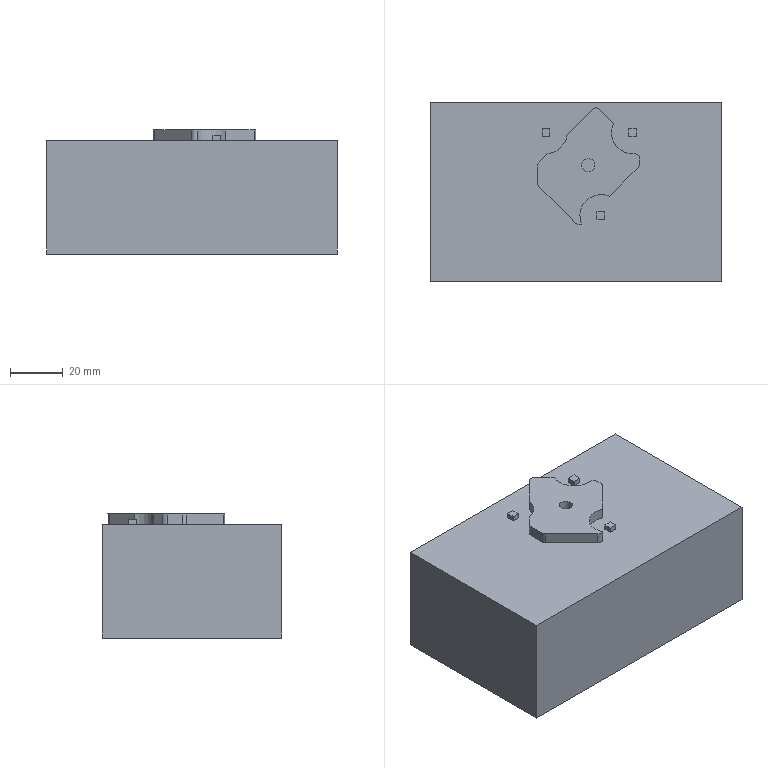CAM job | NX | 3-axis milling, drilling | part box 110.151 x 68.163 x 47.1 mm | stock box 110.151 x 68.163 x 47.1 mm
Tools:
number,name,description,diameter,corner_radius,flute_length,length,flutes
0,D50,Milling Tool-5 Parameters,50.0,0.0,50.0,75.0,2
0,D25R0,Milling Tool-5 Parameters,25.0,0.0,50.0,75.0,2
0,D6R0,Milling Tool-5 Parameters,6.0,0.0,40.0,40.0,2
12,D10R0,Milling Tool-5 Parameters,10.0,0.0,45.0,45.0,2
0,DK-Ø6,Drilling Tool,6.0,0.0,50.0,50.0,2
0,D1.8钻头,Drilling Tool,1.8,0.0,35.0,50.0,2
0,D2.75钻头,Drilling Tool,2.75,0.0,35.0,50.0,2
0,M2,Drilling Tool,2.0,0.0,35.0,50.0,4
0,M3,Drilling Tool,3.0,0.0,35.0,50.0,4
0,D16R0,Milling Tool-5 Parameters,16.0,0.0,50.0,75.0,2
0,D12R0,Milling Tool-5 Parameters,12.0,0.0,50.0,75.0,2
0,D4.2钻头,Drilling Tool,4.2,0.0,35.0,50.0,2
0,DK-Ø8,Countersink,8.0,0.0,0.0,60.0,2
0,D3.4钻头,Drilling Tool,3.4,0.0,35.0,50.0,2
0,M5,Drilling Tool,5.0,0.0,35.0,50.0,4
0,D4R0,Milling Tool-5 Parameters,4.0,0.0,50.0,75.0,2
4,D8R0,Milling Tool-5 Parameters,8.0,0.0,50.0,50.0,2
0,D2R0,Milling Tool-5 Parameters,2.0,0.0,20.0,20.0,2
0,R5,Milling Tool-Ball Mill,10.0,5.0,50.0,75.0,2
0,D3.7钻头,Drilling Tool,3.7,0.0,60.0,60.0,2
0,D5.3钻头,Drilling Tool,5.3,0.0,35.0,50.0,2
0,D3R0,Milling Tool-5 Parameters,3.0,0.0,28.0,28.0,2
0,DJ-Ø5,Countersink,5.0,0.0,0.0,60.0,2
0,DJ-Ø3,Countersink,3.0,0.0,0.0,20.0,2
0,DK-Ø12,Countersink,12.0,0.0,0.0,60.0,2
0,D8.5钻,Drilling Tool,8.5,0.0,35.0,50.0,2
0,D5.5钻,Drilling Tool,5.5,0.0,35.0,50.0,2
0,D6.6钻,Drilling Tool,6.5,0.0,35.0,50.0,2
0,D2.5钻,Drilling Tool,2.5,0.0,35.0,50.0,2
0,D05,Drilling Tool,5.0,0.0,35.0,50.0,2
0,M6,Drilling Tool,6.0,0.0,35.0,50.0,4
0,DK-Ø5,Countersink,5.0,0.0,0.0,60.0,2
0,D02钻头,Drilling Tool,2.0,0.0,35.0,80.0,2
0,M2.50,Drilling Tool,2.5,0.0,35.0,50.0,4
0,D2.5R0,Milling Tool-5 Parameters,2.5,0.0,50.0,75.0,2
0,D1.5R0,Milling Tool-5 Parameters,1.5,0.0,4.5,4.5,2
1,E63,Milling Tool-5 Parameters,63.0,0.0,50.0,75.0,2
0,DD10,Thread Mill,9.95,0.0,10.0,50.0,2
21,D10,Milling Tool-5 Parameters,10.0,0.0,50.0,75.0,2
Operations:
program,operation,operation_type,tool,method,geometry_group,spindle_rpm,surface_speed,feed_per_tooth,feed_cut,feed_plunge,cut_length_mm,path_length_mm,cut_time_min,machine_time_min
A01,FACE_MILLING,FaceMilling,E63,METHOD,MCS_MILL,3000.0,471.0,0.25,1500.0,100.0,413.956,579.956,0.276,0.3009
A01,PLANAR_PROFILE_2,PlanarMilling,E63,METHOD,MCS_MILL,5000.0,989.0,0.18,1800.0,100.0,3196.863,3424.863,1.776,1.807
A01,ZLEVEL_PROFILE_STEEP,ZLevelMilling,E63,METHOD,MCS_MILL,5000.0,100.0,0.1178,3000.0,100.0,8146.876,18371.908,2.716,4.073
A02,FACE_MILLING_1_COPY_1,FaceMilling,D25R0,METHOD,MCS_MILL,6000.0,392.0,0.25,2500.0,100.0,3268.899,3674.908,1.308,1.349
A02,PLANAR_MILL,PlanarMilling,D25R0,METHOD,MCS_MILL,6000.0,392.0,0.25,2500.0,100.0,4270.959,4460.559,1.708,1.736
A02,CAVITY_MILL_4,CavityMilling,D25R0,METHOD,MCS_MILL,6000.0,392.0,0.25,2500.0,100.0,3586.891,3906.091,1.435,1.479
A03,CAVITY_MILL_COPY_COPY,CavityMilling,D10R0,METHOD,MCS_MILL,5000.0,157.0,0.15,1500.0,100.0,915.845,1744.833,0.6106,0.763
A03,CAVITY_MILL,CavityMilling,D10R0,METHOD,MCS_MILL,5000.0,157.0,0.15,1500.0,100.0,1525.257,1761.257,1.017,1.068
A03,CAVITY_MILL_1,CavityMilling,D10R0,METHOD,MCS_MILL,4000.0,125.0,0.1875,1500.0,100.0,1369.169,1660.481,0.9128,0.9541
A04,DRILLING,Operation,DK-Ø8,METHOD,MCS_MILL,2000.0,37.0,0.05,200.0,0.0,12.0,469.097,0.06,0.1057
A04,DRILLING_COPY,Operation,DK-Ø8,METHOD,MCS_MILL,2000.0,37.0,0.05,200.0,0.0,12.0,548.039,0.06,0.1136
A04,DRILLING_COPY_COPY,Operation,DK-Ø8,METHOD,MCS_MILL,2000.0,37.0,0.05,200.0,0.0,6.7,302.057,0.0335,0.063
A04,DRILLING_COPY_COPY_COPY,Operation,DK-Ø8,METHOD,MCS_MILL,2000.0,37.0,0.05,200.0,0.0,11.4,521.628,0.057,0.108
A04,PLANAR_MILL_COPY,PlanarMilling,DK-Ø8,METHOD,MCS_MILL,3500.0,87.0,0.1714,1200.0,100.0,347.153,510.153,0.2893,0.3137
A05,DRILLING_COPY_COPY_COPY_COPY,Operation,D1.8钻头,METHOD,MCS_MILL,1800.0,10.0,0.0278,100.0,0.0,20.0,538.828,0.2,0.2519
A06,DRILLING_COPY_COPY_COPY_1,Operation,D2.75钻头,METHOD,MCS_MILL,2000.0,17.0,0.025,100.0,0.0,23.0,334.657,0.23,0.2612
A07,DRILLING_COPY_COPY_COPY_COPY_COPY,Operation,M2,METHOD,MCS_MILL,300.0,1.0,0.1,120.0,0.0,20.0,538.828,0.1667,0.2185
A08,DRILLING_COPY_COPY_COPY_COPY_COPY_COPY,Operation,M3,METHOD,MCS_MILL,300.0,2.0,0.125,150.0,0.0,17.0,322.657,0.1133,0.1439
A09,PLANAR_MILL_COPY_1,PlanarMilling,D10R0,METHOD,MCS_MILL,4000.0,125.0,0.1,800.0,100.0,369.021,555.321,0.4613,0.4892
B01,FACE_MILLING_COPY,FaceMilling,E63,METHOD,MCS_MILL,3500.0,692.0,0.3571,2500.0,100.0,3199.647,3711.185,1.28,1.339
B02,CAVITY_MILL_2,CavityMilling,D12R0,METHOD,MCS_MILL,5500.0,207.0,0.1364,1500.0,100.0,2703.853,2986.78,1.803,1.852
B03,PLANAR_MILL_2_COPY,PlanarMilling,D10R0,METHOD,MCS_MILL,4000.0,125.0,0.1,800.0,100.0,824.431,984.431,1.03,1.054
B03,CAVITY_MILL_2_COPY_1,CavityMilling,D10R0,METHOD,MCS_MILL,4500.0,141.0,0.0889,800.0,100.0,821.409,992.209,1.027,1.064
B04,DRILLING_COPY_COPY_COPY_COPY_1,Operation,DK-Ø8,METHOD,MCS_MILL,2000.0,37.0,0.05,200.0,0.0,11.1,457.326,0.0555,0.1001
B04,DRILLING_COPY_COPY_COPY_COPY_1_COPY_1,Operation,DK-Ø8,METHOD,MCS_MILL,2000.0,50.0,0.0375,150.0,0.0,18.0,560.039,0.12,0.1742
B04,PLANAR_MILL_COPY_COPY,PlanarMilling,DK-Ø8,METHOD,MCS_MILL,4000.0,100.0,0.15,1200.0,100.0,135.803,299.803,0.1132,0.1378
B04,PLANAR_MILL_COPY_COPY_COPY,PlanarMilling,DK-Ø8,METHOD,MCS_MILL,4000.0,100.0,0.15,1200.0,100.0,443.823,607.823,0.3699,0.3945
B04,DRILLING_COPY_COPY_COPY_COPY_1_COPY_2,Operation,DK-Ø8,METHOD,MCS_MILL,2000.0,37.0,0.05,200.0,0.0,8.4,310.48,0.042,0.0722
B05,DRILLING_COPY_COPY_COPY_COPY_1_COPY,Operation,D4.2钻头,METHOD,MCS_MILL,1800.0,23.0,0.0556,200.0,0.0,52.5,540.126,0.2625,0.3113
B05,DRILLING_COPY_COPY_COPY_COPY_1_COPY_COPY_2,Operation,D4.2钻头,METHOD,MCS_MILL,1800.0,23.0,0.0556,200.0,0.0,29.0,351.68,0.145,0.1773
B06,DRILLING_COPY_COPY_COPY_COPY_1_COPY_COPY,Operation,D3.4钻头,METHOD,MCS_MILL,1800.0,23.0,0.0556,200.0,0.0,30.0,584.039,0.15,0.2054
B07,DRILLING_COPY_COPY_COPY_COPY_1_COPY_COPY_1,Operation,M5,METHOD,MCS_MILL,400.0,6.0,0.2,320.0,0.0,43.5,522.126,0.1359,0.1838
B08,PLANAR_MILL_2,PlanarMilling,D4R0,METHOD,MCS_MILL,5000.0,62.0,0.15,1500.0,100.0,814.97,1251.944,0.5433,0.6029
B08,PLANAR_MILL_2_COPY_1,PlanarMilling,D4R0,METHOD,MCS_MILL,4000.0,50.0,0.025,200.0,100.0,31.176,479.723,0.1559,0.2183
B08,PLANAR_MILL_2_COPY_1_COPY,PlanarMilling,D4R0,METHOD,MCS_MILL,4000.0,50.0,0.025,200.0,100.0,31.176,479.723,0.1559,0.2183
B-5,PLANAR_MILL_2_COPY_COPY_1,PlanarMilling,D10R0,METHOD,MCS_MILL,4000.0,125.0,0.1,800.0,100.0,824.431,984.431,1.03,1.054
C01,DRILLING_1,Operation,DK-Ø5,METHOD,MCS_MILL,1500.0,23.0,0.05,150.0,0.0,4.0,108.0,0.0267,0.0371
C01,DRILLING_1_COPY,Operation,DK-Ø5,METHOD,MCS_MILL,1800.0,28.0,0.0417,150.0,0.0,3.5,107.0,0.0233,0.0337
C01,DRILLING_1_COPY_1,Operation,D3.7钻头,METHOD,MCS_MILL,1800.0,20.0,0.0417,150.0,0.0,22.5,145.0,0.15,0.1622
C01,DRILLING_1_COPY_COPY,Operation,D3.7钻头,METHOD,MCS_MILL,1800.0,20.0,0.0417,150.0,0.0,19.5,139.0,0.13,0.1419
C01,DRILLING_1_COPY_1_COPY,Operation,D5.3钻头,METHOD,MCS_MILL,1500.0,21.0,0.0667,200.0,0.0,11.5,123.0,0.0575,0.0687
C01,PLANAR_MILL_3_COPY_3,PlanarMilling,D8R0,METHOD,MCS_MILL,5000.0,125.0,0.1,1000.0,1500.0,239.323,604.823,0.2325,0.3
C01,PLANAR_MILL_3_COPY_3_COPY_2,PlanarMilling,D8R0,METHOD,MCS_MILL,5500.0,138.0,0.0909,1000.0,1500.0,70.885,686.617,0.0605,0.1839
C01,PLANAR_MILL_3_COPY_3_COPY,PlanarMilling,D8R0,METHOD,MCS_MILL,5500.0,138.0,0.0909,1000.0,1500.0,209.6,673.919,0.2027,0.2849
C01,PLANAR_MILL_3_COPY_3_COPY_COPY_1,PlanarMilling,D8R0,METHOD,MCS_MILL,5500.0,138.0,0.0909,1000.0,1500.0,209.6,673.919,0.2027,0.2849
C01,PLANAR_MILL_3_COPY_3_COPY_COPY,PlanarMilling,D8R0,METHOD,MCS_MILL,5500.0,138.0,0.0727,800.0,1500.0,104.8,340.319,0.1249,0.1698
C01,CAVITY_MILL_COPY_1_COPY,CavityMilling,D8R0,METHOD,MCS_MILL,5500.0,138.0,0.2273,2500.0,1500.0,2374.209,2588.138,0.9691,1.01
C01,PLANAR_PROFILE_COPY,PlanarMilling,D8R0,METHOD,MCS_MILL,5500.0,138.0,0.0909,1000.0,1500.0,79.287,154.488,0.0774,0.0887
C01,PLANAR_PROFILE_COPY_COPY,PlanarMilling,D8R0,METHOD,MCS_MILL,5500.0,138.0,0.0591,650.0,1500.0,91.316,166.516,0.1355,0.1468
C01,PLANAR_MILL_4,PlanarMilling,D6R0,METHOD,MCS_MILL,6500.0,122.0,0.1923,2500.0,100.0,723.805,899.003,0.2895,0.3151
C01,PLANAR_MILL_4_COPY,PlanarMilling,D6R0,METHOD,MCS_MILL,6500.0,122.0,0.0615,800.0,100.0,90.876,258.876,0.1136,0.1388
C01,PLANAR_MILL_3_COPY_3_COPY_COPY_COPY_COPY,PlanarMilling,D10,METHOD,MCS_MILL,3000.0,94.0,0.1333,800.0,1500.0,55.0,182.119,0.065,0.0925
C01,PLANAR_MILL_3_COPY_3_COPY_1,PlanarMilling,D10,METHOD,MCS_MILL,5000.0,125.0,0.1,1000.0,1500.0,86.159,221.459,0.0833,0.1126
C01,PLANAR_MILL_3_COPY_3_COPY_1_COPY_1,PlanarMilling,D10,METHOD,MCS_MILL,5000.0,125.0,0.1,1000.0,1500.0,86.159,221.459,0.0833,0.1126
C01,PLANAR_PROFILE_1,PlanarMilling,D10R0,METHOD,MCS_MILL,4500.0,141.0,0.0889,800.0,100.0,57.0,97.0,0.0713,0.0773
C01,PLANAR_PROFILE_1_COPY,PlanarMilling,D10R0,METHOD,MCS_MILL,4000.0,125.0,0.25,2000.0,100.0,676.096,1478.598,0.338,0.4314
C01,PLANAR_PROFILE_1_COPY_COPY,PlanarMilling,D10R0,METHOD,MCS_MILL,4000.0,125.0,0.05,400.0,100.0,67.498,186.298,0.3612,0.3791
C01,CAVITY_MILL_5,CavityMilling,D10R0,METHOD,MCS_MILL,4500.0,141.0,0.2222,2000.0,1000.0,2268.244,2661.886,1.298,1.347
C01,PLANAR_MILL_3_COPY_3_COPY_1_COPY,PlanarMilling,D10R0,METHOD,MCS_MILL,4000.0,125.0,0.1,800.0,100.0,49.615,173.471,0.062,0.0889
C01,CAVITY_MILL_COPY_1,CavityMilling,D10R0,METHOD,MCS_MILL,4000.0,125.0,0.1875,1500.0,100.0,953.266,2865.225,0.6355,0.9772
C01,FACE_MILLING_2,FaceMilling,D10R0,METHOD,MCS_MILL,4000.0,125.0,0.05,400.0,100.0,15.0,120.9,0.0375,0.0534
C01,PLANAR_MILL_3_COPY_4,PlanarMilling,D10R0,METHOD,MCS_MILL,4000.0,125.0,0.05,400.0,100.0,15.0,115.0,0.0375,0.0592
C01,PLANAR_MILL_3_COPY_4_COPY,PlanarMilling,D10R0,METHOD,MCS_MILL,4000.0,125.0,0.05,400.0,100.0,15.0,115.0,0.0375,0.0592
C01,PLANAR_MILL_3_COPY_4_COPY_COPY,PlanarMilling,D10R0,METHOD,MCS_MILL,4000.0,125.0,0.05,400.0,100.0,13.0,115.3,0.0325,0.0547
C01,PLANAR_MILL_3_COPY_3_COPY_COPY_1_COPY_COPY,PlanarMilling,R5,METHOD,MCS_MILL,4500.0,141.0,0.0444,400.0,1500.0,57.0,172.6,0.1288,0.1538
C01,CAVITY_MILL_COPY_1_COPY_COPY,CavityMilling,D4R0,METHOD,MCS_MILL,3000.0,37.0,0.25,1500.0,100.0,918.512,2163.766,0.6123,0.8259
C01,CAVITY_MILL_COPY_1_COPY_COPY_COPY,CavityMilling,D4R0,METHOD,MCS_MILL,3000.0,37.0,0.0667,400.0,100.0,94.513,223.713,0.2363,0.2643
C01,CAVITY_MILL_COPY_1_COPY_COPY_COPY_COPY,CavityMilling,D4R0,METHOD,MCS_MILL,3000.0,37.0,0.0667,400.0,100.0,94.513,223.713,0.2363,0.2643
C01,CAVITY_MILL_COPY_1_COPY_COPY_COPY_COPY_COPY,CavityMilling,D4R0,METHOD,MCS_MILL,3000.0,37.0,0.0667,400.0,100.0,94.513,223.713,0.2363,0.2643
C01,PLANAR_MILL_5,PlanarMilling,D3R0,METHOD,MCS_MILL,3500.0,32.0,0.2857,2000.0,100.0,1535.272,1640.072,0.7676,0.7831
C01,PLANAR_MILL_5_COPY,PlanarMilling,D3R0,METHOD,MCS_MILL,3000.0,28.0,0.25,1500.0,100.0,387.795,488.795,0.2585,0.2736
C01,PLANAR_MILL_5_COPY_COPY,PlanarMilling,D3R0,METHOD,MCS_MILL,3000.0,28.0,0.25,1500.0,100.0,1019.419,1125.119,0.6796,0.6952
C01,PLANAR_MILL_5_COPY_1,PlanarMilling,D3R0,METHOD,MCS_MILL,3000.0,28.0,0.05,300.0,100.0,128.642,233.542,0.4288,0.4445
C01,PLANAR_MILL_5_COPY_COPY_1,PlanarMilling,D3R0,METHOD,MCS_MILL,3000.0,28.0,0.05,300.0,100.0,129.768,230.868,0.4326,0.4477
C01,PLANAR_MILL_5_COPY_COPY_COPY_1,PlanarMilling,D3R0,METHOD,MCS_MILL,4000.0,37.0,0.05,400.0,100.0,101.608,204.608,0.254,0.2695
C01,PLANAR_MILL_5_COPY_COPY_COPY,PlanarMilling,D2R0,METHOD,MCS_MILL,5000.0,31.0,0.1,1000.0,100.0,313.795,1097.954,0.3138,0.4223
C01,PLANAR_MILL_5_COPY_2_COPY_2,PlanarMilling,DJ-Ø5,METHOD,MCS_MILL,4000.0,62.0,0.125,1000.0,100.0,132.795,296.795,0.1328,0.1574
C01,PLANAR_MILL_5_COPY_2_COPY,PlanarMilling,DJ-Ø5,METHOD,MCS_MILL,4000.0,62.0,0.125,1000.0,100.0,254.474,416.474,0.2545,0.2788
C01,PLANAR_MILL_5_COPY_2_COPY_COPY,PlanarMilling,DJ-Ø5,METHOD,MCS_MILL,4000.0,62.0,0.125,1000.0,100.0,21.283,183.283,0.0213,0.0456
C01,PLANAR_MILL_5_COPY_2_COPY_1,PlanarMilling,DJ-Ø5,METHOD,MCS_MILL,4000.0,62.0,0.125,1000.0,100.0,103.562,165.562,0.1036,0.1129
C01,PLANAR_MILL_5_COPY_2_COPY_COPY_COPY,PlanarMilling,DJ-Ø5,METHOD,MCS_MILL,4000.0,62.0,0.125,1000.0,100.0,40.053,281.928,0.0401,0.0744
C01,DRILLING_1_COPY_COPY_1,Operation,DJ-Ø5,METHOD,MCS_MILL,2000.0,31.0,0.025,100.0,0.0,12.4,573.031,0.124,0.1801
C01,DRILLING_1_COPY_COPY_3,Operation,DK-Ø5,METHOD,MCS_MILL,1800.0,28.0,0.0417,150.0,0.0,3.5,123.0,0.0233,0.0353
C01,PLANAR_MILL_3_COPY_5,PlanarMilling,D10R0,METHOD,MCS_MILL,4500.0,141.0,0.0667,600.0,1500.0,212.847,372.847,0.3443,0.379
C01,PLANAR_MILL_3_COPY_COPY,PlanarMilling,D10R0,METHOD,MCS_MILL,4500.0,141.0,0.0722,650.0,1500.0,99.417,265.417,0.1488,0.1848
C01,PLANAR_MILL_3_COPY_1_COPY_COPY,PlanarMilling,D10R0,METHOD,MCS_MILL,4500.0,141.0,0.0667,600.0,1500.0,196.762,359.922,0.3175,0.3529
C01,PLANAR_MILL_3_COPY_2_COPY_COPY,PlanarMilling,D10R0,METHOD,MCS_MILL,4500.0,141.0,0.0667,600.0,1500.0,184.007,356.007,0.2963,0.3335
C01,D10燕尾刀,PlanarMilling,D10R0,METHOD,MCS_MILL,6000.0,188.0,0.0667,800.0,100.0,197.01,358.698,0.2463,0.2704
C01,PLANAR_MILL_3_COPY_3_COPY_1_COPY_1_COPY,PlanarMilling,D8R0,METHOD,MCS_MILL,3500.0,87.0,0.0571,300.0,100.0,70.64,150.54,0.2355,0.2528
C01,THREAD_MILLING,ThreadMilling,DD10,METHOD,MCS_MILL,5000.0,155.0,0.04,400.0,100.0,485.462,652.491,1.214,1.23
C01,PLANAR_MILL_3,PlanarMilling,DJ-Ø3,METHOD,MCS_MILL,4000.0,37.0,0.1,800.0,100.0,120.498,278.498,0.1506,0.1664
C01,PLANAR_MILL_3_COPY,PlanarMilling,DJ-Ø3,METHOD,MCS_MILL,4000.0,37.0,0.1,800.0,100.0,114.233,272.233,0.1428,0.1586
C01,PLANAR_MILL_5_COPY_2_COPY_COPY_COPY_COPY,PlanarMilling,DJ-Ø3,METHOD,MCS_MILL,4000.0,37.0,0.05,400.0,100.0,210.599,312.799,0.5265,0.5418
C01,PLANAR_MILL_5_COPY_2_COPY_COPY_COPY_COPY_COPY,PlanarMilling,DJ-Ø3,METHOD,MCS_MILL,4000.0,37.0,0.05,400.0,100.0,107.962,210.162,0.2699,0.2852
C01,PLANAR_MILL_5_COPY_3_COPY_1,PlanarMilling,D3R0,METHOD,MCS_MILL,4000.0,37.0,0.05,400.0,100.0,221.318,392.745,0.5533,0.5784
C01,PLANAR_MILL_5_COPY_3_COPY_COPY,PlanarMilling,D3R0,METHOD,MCS_MILL,4000.0,37.0,0.05,400.0,100.0,174.956,343.956,0.4374,0.4623
C01,PLANAR_MILL_5_COPY_3_COPY_COPY_COPY_COPY_COPY,PlanarMilling,D3R0,METHOD,MCS_MILL,3000.0,28.0,0.0133,80.0,100.0,18.281,194.281,0.2285,0.2549
C01,PLANAR_MILL_5_COPY_3_COPY_1_COPY_1_COPY,PlanarMilling,D3R0,METHOD,MCS_MILL,3000.0,28.0,0.0133,80.0,100.0,18.306,201.159,0.2288,0.2563
C01,FLOOR_WALL_3_COPY_COPY_COPY,VolumeBased25DMillingOperation,D10R0,METHOD,MCS_MILL,3500.0,109.0,0.0857,600.0,100.0,1075.962,2001.095,1.793,1.911
C01,FLOOR_WALL_3_COPY_COPY,VolumeBased25DMillingOperation,D10R0,METHOD,MCS_MILL,3500.0,109.0,0.0857,600.0,100.0,1075.962,2009.083,1.793,1.912
C01,FACE_MILLING_2_COPY,FaceMilling,D10R0,METHOD,MCS_MILL,4000.0,125.0,0.125,1000.0,100.0,15.0,120.86,0.015,0.0309
C01,PLANAR_MILL_3_COPY_4_COPY_1_COPY,PlanarMilling,D10R0,METHOD,MCS_MILL,4500.0,141.0,0.0444,400.0,1500.0,15.0,115.0,0.0265,0.0482
C01,PLANAR_MILL_3_COPY_4_COPY_COPY_1_COPY,PlanarMilling,D10R0,METHOD,MCS_MILL,4500.0,141.0,0.0444,400.0,1500.0,15.0,115.0,0.0265,0.0482
C01,PLANAR_MILL_3_COPY_4_COPY_COPY_COPY_COPY_1,PlanarMilling,D10R0,METHOD,MCS_MILL,4500.0,141.0,0.0444,400.0,1500.0,13.0,115.34,0.0233,0.0455
C01,PLANAR_MILL_3_COPY_4_COPY_1_COPY_COPY,PlanarMilling,D10R0,METHOD,MCS_MILL,6500.0,204.0,0.0308,400.0,1500.0,15.0,115.0,0.0265,0.0482
C01,PLANAR_MILL_3_COPY_4_COPY_COPY_1_COPY_COPY,PlanarMilling,D10R0,METHOD,MCS_MILL,6500.0,204.0,0.0308,400.0,1500.0,15.0,115.0,0.0265,0.0482
C01,PLANAR_MILL_3_COPY_4_COPY_COPY_COPY_COPY_1_COPY_1,PlanarMilling,D10R0,METHOD,MCS_MILL,6500.0,204.0,0.0308,400.0,1500.0,13.0,115.36,0.0233,0.0455
C01,PLANAR_MILL_3_COPY_4_COPY_COPY_COPY_COPY_1_COPY,PlanarMilling,D10R0,METHOD,MCS_MILL,3000.0,94.0,0.1,600.0,1500.0,217.2,2345.48,0.302,0.7359
C01,PLANAR_MILL_3_COPY_4_COPY_COPY_COPY_COPY_COPY,PlanarMilling,D10R0,METHOD,MCS_MILL,3000.0,141.0,0.0667,600.0,1500.0,52.0,227.89,0.0817,0.1198
C01,PLANAR_MILL_3_COPY_4_COPY_COPY_COPY_COPY_COPY_COPY,PlanarMilling,D10R0,METHOD,MCS_MILL,3000.0,141.0,0.0667,600.0,1500.0,84.296,396.438,0.1305,0.185
D01,PLANAR_MILL_2_COPY_COPY,PlanarMilling,D10R0,METHOD,MCS_MILL,5000.0,157.0,0.2,2000.0,100.0,422.849,462.849,0.2114,0.2174
D01,PLANAR_MILL_2_COPY_COPY_COPY,PlanarMilling,D10R0,METHOD,MCS_MILL,5000.0,157.0,0.2,2000.0,100.0,63.946,103.946,0.032,0.038
D01,PLANAR_PROFILE,PlanarMilling,D10R0,METHOD,MCS_MILL,5000.0,157.0,0.2,2000.0,100.0,698.8,757,0.3494,0.3573
D01,PLANAR_PROFILE_COPY_2,PlanarMilling,D10R0,METHOD,MCS_MILL,5000.0,157.0,0.2,2000.0,100.0,1493.358,1551.558,0.7467,0.7546
D01,CAVITY_MILL_2_COPY,CavityMilling,D10R0,METHOD,MCS_MILL,5000.0,157.0,0.2,2000.0,100.0,712.062,757.062,0.356,0.3652
D01,CAVITY_MILL_2_COPY_COPY_COPY,CavityMilling,D10R0,METHOD,MCS_MILL,5000.0,157.0,0.2,2000.0,100.0,537.415,724.515,0.2687,0.3008
D01,PLANAR_MILL_COPY_1_1,PlanarMilling,D1.5R0,METHOD,MCS_MILL,6000.0,28.0,0.1,1200.0,100.0,982.84,1025.54,0.819,0.8253
D01,PLANAR_MILL_COPY_1_COPY,PlanarMilling,D1.5R0,METHOD,MCS_MILL,6000.0,33.0,0.0667,800.0,100.0,430.497,471.297,0.5381,0.5442
D01,PLANAR_MILL_1_1,PlanarMilling,D1.5R0,METHOD,MCS_MILL,6000.0,28.0,0.125,1500.0,100.0,3038.746,3711.707,2.026,2.101
D01,PLANAR_MILL_1_1_COPY,PlanarMilling,D1.5R0,METHOD,MCS_MILL,5500.0,25.0,0.0364,400.0,100.0,98.781,268.063,0.247,0.2723
D01,DRILLING_COPY_1,Operation,DK-Ø6,METHOD,MCS_MILL,2000.0,31.0,0.025,100.0,0.0,2.25,64.5,0.0225,0.0287
D01,DRILLING_COPY_1_COPY,Operation,DK-Ø6,METHOD,MCS_MILL,2000.0,31.0,0.025,100.0,0.0,2.25,64.5,0.0225,0.0287
D01,DRILLING_COPY_1_COPY_COPY_2,Operation,DK-Ø6,METHOD,MCS_MILL,2000.0,31.0,0.025,100.0,0.0,3.5,67.0,0.035,0.0414
D01,DRILLING_COPY_1_COPY_COPY_2_COPY,Operation,DK-Ø6,METHOD,MCS_MILL,2000.0,31.0,0.025,100.0,0.0,3.0,66.0,0.03,0.0363
D01,PLANAR_PROFILE_COPY_3,PlanarMilling,DK-Ø6,METHOD,MCS_MILL,4000.0,62.0,0.125,1000.0,100.0,381.698,423.698,0.3817,0.388
D01,PLANAR_PROFILE_COPY_3_COPY,PlanarMilling,DK-Ø6,METHOD,MCS_MILL,4000.0,62.0,0.125,1000.0,100.0,123.858,165.857,0.1239,0.1302
D01,PLANAR_PROFILE_COPY_3_COPY_COPY,PlanarMilling,DK-Ø6,METHOD,MCS_MILL,4000.0,62.0,0.125,1000.0,100.0,31.962,74.962,0.032,0.0384
D01,PLANAR_PROFILE_COPY_3_COPY_COPY_COPY,PlanarMilling,DK-Ø6,METHOD,MCS_MILL,4000.0,62.0,0.125,1000.0,100.0,24.5,67.5,0.0245,0.031
D01,PLANAR_PROFILE_COPY_3_COPY_COPY_1,PlanarMilling,DK-Ø6,METHOD,MCS_MILL,4000.0,62.0,0.125,1000.0,100.0,109.035,150.235,0.109,0.1152
D01,PLANAR_PROFILE_COPY_3_COPY_COPY_2,PlanarMilling,DK-Ø6,METHOD,MCS_MILL,4000.0,62.0,0.125,1000.0,100.0,40.142,81.142,0.0401,0.0463
D01,DRILLING_COPY_1_COPY_1,Operation,D02钻头,METHOD,MCS_MILL,1200.0,7.0,0.0417,100.0,0.0,31.0,122.0,0.31,0.3191
D01,DRILLING_COPY_1_COPY_COPY,Operation,D02钻头,METHOD,MCS_MILL,1200.0,7.0,0.0417,100.0,0.0,31.0,122.0,0.31,0.3191
D01,PLANAR_MILL_8,PlanarMilling,D2.5R0,METHOD,MCS_MILL,6000.0,47.0,0.0667,800.0,100.0,185.922,231.622,0.2324,0.2389
D01,PLANAR_MILL_COPY_2,PlanarMilling,D2.5R0,METHOD,MCS_MILL,6000.0,47.0,0.0417,500.0,100.0,59.901,101.341,0.1198,0.1259
D01,DRILLING_COPY_1_COPY_1_COPY,Operation,M2.50,METHOD,MCS_MILL,200.0,1.0,0.1125,90.0,0.0,6.0,72.0,0.0667,0.0733
D01,DRILLING_COPY_1_COPY_COPY_COPY,Operation,M2.50,METHOD,MCS_MILL,200.0,1.0,0.1125,90.0,0.0,6.0,72.0,0.0667,0.0733
D01,DRILLING_COPY_1_COPY_COPY_1,Operation,M5,METHOD,MCS_MILL,400.0,6.0,0.2,320.0,0.0,7.3,74.6,0.0228,0.0295
D01,PLANAR_MILL_2_COPY_COPY_COPY_1,PlanarMilling,D10R0,METHOD,MCS_MILL,5000.0,157.0,0.08,800.0,100.0,425.479,465.479,0.5318,0.5378
D01,PLANAR_MILL_2_COPY_COPY_COPY_COPY,PlanarMilling,D10R0,METHOD,MCS_MILL,4500.0,141.0,0.0889,800.0,100.0,60.946,100.946,0.0762,0.0822
D01,CAVITY_MILL_2_COPY_COPY_1_COPY_1,CavityMilling,D10R0,METHOD,MCS_MILL,4500.0,141.0,0.0889,800.0,100.0,1004.466,1217.66,1.256,1.29
D01,PLANAR_PROFILE_COPY_4,PlanarMilling,D10R0,METHOD,MCS_MILL,4500.0,141.0,0.0722,650.0,100.0,69.644,127.844,0.1071,0.1159
D01,PLANAR_PROFILE_COPY_2_COPY,PlanarMilling,D10R0,METHOD,MCS_MILL,4500.0,141.0,0.0722,650.0,100.0,148.864,207.065,0.229,0.2378
O0001.NC,PLANAR_MILL_2_COPY_COPY_COPY_2,PlanarMilling,D10R0,METHOD,MCS_MILL,5000.0,157.0,0.2,2000.0,100.0,422.849,462.849,0.2114,0.2174
O0001.NC,PLANAR_MILL_2_COPY_COPY_COPY_COPY_1,PlanarMilling,D10R0,METHOD,MCS_MILL,5000.0,157.0,0.2,2000.0,100.0,63.946,103.946,0.032,0.038
O0001.NC,PLANAR_PROFILE_COPY_1,PlanarMilling,D10R0,METHOD,MCS_MILL,5000.0,157.0,0.2,2000.0,100.0,698.015,756.215,0.349,0.3569
O0001.NC,PLANAR_PROFILE_COPY_2_COPY_1,PlanarMilling,D10R0,METHOD,MCS_MILL,5000.0,157.0,0.2,2000.0,100.0,1491.787,1549.987,0.7459,0.7538
O0001.NC,CAVITY_MILL_2_COPY_COPY,CavityMilling,D10R0,METHOD,MCS_MILL,5000.0,157.0,0.2,2000.0,100.0,712.062,757.062,0.356,0.3652
O0001.NC,CAVITY_MILL_2_COPY_COPY_COPY_COPY,CavityMilling,D10R0,METHOD,MCS_MILL,5000.0,157.0,0.2,2000.0,100.0,537.415,724.515,0.2687,0.3008
O0001.NC,PLANAR_MILL_2_COPY_COPY_COPY_1_COPY,PlanarMilling,D10R0,METHOD,MCS_MILL,5000.0,157.0,0.08,800.0,100.0,425.479,465.479,0.5318,0.5378
O0001.NC,PLANAR_MILL_2_COPY_COPY_COPY_COPY_COPY,PlanarMilling,D10R0,METHOD,MCS_MILL,4500.0,141.0,0.0889,800.0,100.0,60.946,100.946,0.0762,0.0822
O0001.NC,CAVITY_MILL_2_COPY_COPY_1_COPY_1_COPY,CavityMilling,D10R0,METHOD,MCS_MILL,4500.0,141.0,0.0889,800.0,100.0,1004.466,1217.66,1.256,1.29
O0001.NC,PLANAR_PROFILE_COPY_4_COPY,PlanarMilling,D10R0,METHOD,MCS_MILL,4500.0,141.0,0.0722,650.0,100.0,69.644,127.844,0.1071,0.1159
O0001.NC,PLANAR_PROFILE_COPY_2_COPY_COPY,PlanarMilling,D10R0,METHOD,MCS_MILL,4500.0,141.0,0.0722,650.0,100.0,148.864,207.065,0.229,0.2378
O0001.NC,PLANAR_PROFILE_COPY_3_COPY_COPY_3_COPY,PlanarMilling,D10R0,METHOD,MCS_MILL,4000.0,62.0,0.125,1000.0,100.0,83.897,134.097,0.0839,0.0914
O0001.NC,PLANAR_PROFILE_COPY_3_COPY_COPY_3_COPY_COPY,PlanarMilling,D10R0,METHOD,MCS_MILL,4000.0,62.0,0.125,800.0,100.0,83.897,134.097,0.1049,0.1124
O0001.NC,PLANAR_PROFILE_COPY_3_COPY_1,PlanarMilling,DK-Ø6,METHOD,MCS_MILL,4000.0,62.0,0.125,1000.0,100.0,381.698,423.698,0.3817,0.388
O0001.NC,PLANAR_PROFILE_COPY_3_COPY_COPY_3,PlanarMilling,DK-Ø6,METHOD,MCS_MILL,4000.0,62.0,0.125,1000.0,100.0,123.858,165.857,0.1239,0.1302
O0001.NC,PLANAR_PROFILE_COPY_3_COPY_COPY_COPY_1,PlanarMilling,DK-Ø6,METHOD,MCS_MILL,4000.0,62.0,0.125,1000.0,100.0,31.962,74.962,0.032,0.0384
O0001.NC,PLANAR_PROFILE_COPY_3_COPY_COPY_COPY_COPY,PlanarMilling,DK-Ø6,METHOD,MCS_MILL,4000.0,62.0,0.125,1000.0,100.0,24.5,67.5,0.0245,0.031
O0001.NC,DRILLING_COPY_1_COPY_2,Operation,DK-Ø6,METHOD,MCS_MILL,2000.0,31.0,0.025,100.0,0.0,4.5,194.427,0.045,0.064
1,FACE_MILLING_COPY_1,FaceMilling,D50,METHOD,MCS_MILL,3000.0,471.0,0.1667,1000.0,100.0,454.022,620.023,0.454,0.4789
1,PLANAR_MILL_1,PlanarMilling,D16R0,METHOD,MCS_MILL,4500.0,226.0,0.1667,1500.0,100.0,9544.266,10003.437,6.363,6.417
1,PLANAR_MILL_1_COPY,PlanarMilling,D16R0,METHOD,MCS_MILL,3500.0,175.0,0.0571,400.0,100.0,559.027,799.627,1.398,1.434
1,PLANAR_MILL_1_COPY_COPY,PlanarMilling,D16R0,METHOD,MCS_MILL,3500.0,175.0,0.0571,400.0,100.0,559.027,799.627,1.398,1.434
1,DRILLING_2,Operation,DK-Ø12,METHOD,NONE,2000.0,75.0,0.0375,150.0,0.0,24.0,597.151,0.16,0.2173
1,DRILLING_2_COPY,Operation,DK-Ø12,METHOD,NONE,2000.0,75.0,0.0375,150.0,0.0,21.0,442.484,0.14,0.1821
1,DRILLING_2_COPY_1,Operation,DK-Ø12,METHOD,NONE,2000.0,75.0,0.0375,150.0,0.0,12.0,259.212,0.08,0.1047
1,PLANAR_MILL_1_COPY_COPY_1,PlanarMilling,DK-Ø12,METHOD,MCS_MILL,3500.0,131.0,0.1714,1200.0,100.0,501.427,665.427,0.4179,0.4425
1,DRILLING_2_COPY_2,Operation,D8.5钻,METHOD,NONE,1500.0,40.0,0.05,150.0,0.0,146.0,841.151,0.9733,1.043
1,DRILLING_2_COPY_2_COPY,Operation,D8.5钻,METHOD,NONE,1500.0,40.0,0.05,150.0,0.0,61.5,513.442,0.41,0.4552
1,DRILLING_2_COPY_2_COPY_COPY,Operation,D5.5钻,METHOD,NONE,1500.0,40.0,0.05,150.0,0.0,135.0,660.442,0.9,0.9525
1,DRILLING_2_COPY_2_COPY_COPY_COPY,Operation,D5.5钻,METHOD,NONE,1500.0,40.0,0.05,150.0,0.0,34.0,303.212,0.2267,0.2536
1,DRILLING_2_COPY_2_COPY_COPY_1,Operation,D10R0,METHOD,NONE,1000.0,31.0,0.05,100.0,0.0,58.5,507.442,0.585,0.6299
1,PLANAR_MILL_1_COPY_1,PlanarMilling,D6R0,METHOD,MCS_MILL,5500.0,103.0,0.0727,800.0,100.0,807.102,1216.6,1.009,1.066
2,PLANAR_MILL_1_COPY_1_COPY,PlanarMilling,D6R0,METHOD,MCS_MILL,5500.0,103.0,0.0091,100.0,100.0,15.938,445.338,0.1594,0.2203
2,PLANAR_MILL_1_COPY_1_COPY_COPY,PlanarMilling,D6R0,METHOD,MCS_MILL,5500.0,103.0,0.0091,100.0,100.0,15.938,445.338,0.1594,0.2203
5,FACE_MILLING_COPY_1_COPY,FaceMilling,D50,METHOD,MCS_MILL,4500.0,706.0,0.3889,3500.0,100.0,454.022,624.423,0.1297,0.1553
5,FLOOR_WALL,VolumeBased25DMillingOperation,D16R0,METHOD,MCS_MILL,4500.0,226.0,0.2222,2000.0,100.0,2760.275,3404.434,1.38,1.461
5,FLOOR_WALL_1_COPY,VolumeBased25DMillingOperation,D16R0,METHOD,MCS_MILL,4500.0,226.0,0.1667,1500.0,100.0,942.016,1108.016,0.628,0.6529
5,FLOOR_WALL_COPY,VolumeBased25DMillingOperation,D16R0,METHOD,MCS_MILL,4500.0,226.0,0.0444,400.0,100.0,456.646,1000.453,1.142,1.214
5,FLOOR_WALL_1,VolumeBased25DMillingOperation,D16R0,METHOD,MCS_MILL,4500.0,226.0,0.0667,600.0,100.0,943.321,989.321,1.572,1.579
5,PLANAR_MILL_1_COPY_1_COPY_1_COPY_1,PlanarMilling,D6R0,METHOD,MCS_MILL,5500.0,103.0,0.0727,800.0,100.0,1659.041,2593.151,2.074,2.199
5,PLANAR_MILL_1_COPY_1_COPY_1_COPY_1_COPY,PlanarMilling,D6R0,METHOD,MCS_MILL,5500.0,103.0,0.0182,200.0,100.0,132.531,1106.857,0.6627,0.7961
5,PLANAR_MILL_1_COPY_COPY_1_COPY,PlanarMilling,DK-Ø12,METHOD,MCS_MILL,3500.0,131.0,0.1714,1200.0,100.0,207.926,688.077,0.1733,0.2377
5,PLANAR_MILL_1_COPY_COPY_1_COPY_COPY,PlanarMilling,DK-Ø12,METHOD,MCS_MILL,3500.0,131.0,0.1714,1200.0,100.0,423.827,587.827,0.3532,0.3778
5,DRILLING_2_COPY_2_COPY_COPY_COPY_1_COPY,Operation,DK-Ø12,METHOD,NONE,1500.0,40.0,0.05,150.0,0.0,9.0,277.465,0.06,0.0868
5,PLANAR_TEXT,Engraving,DK-Ø12,METHOD,MCS_MILL,4000.0,37.0,0.0375,300.0,100.0,466.887,1342.411,1.556,1.687
5,DRILLING_2_COPY_2_COPY_COPY_COPY_1,Operation,D5.5钻,METHOD,NONE,1500.0,40.0,0.05,150.0,0.0,37.0,333.465,0.2467,0.2763
5,PLANAR_MILL_1_COPY_1_COPY_1,PlanarMilling,D4R0,METHOD,MCS_MILL,5500.0,103.0,0.0727,800.0,100.0,1765.45,2210.43,2.207,2.267
30,FACE_MILLING_COPY_1_COPY_1,FaceMilling,D50,METHOD,MCS_MILL,3000.0,471.0,0.1667,1000.0,100.0,341.356,507.356,0.3414,0.3663
30,PLANAR_MILL_1_COPY_2,PlanarMilling,D16R0,METHOD,MCS_MILL,4500.0,226.0,0.2778,2500.0,100.0,6646.839,7088.203,2.659,2.711
30,PLANAR_MILL_1_COPY_COPY_2,PlanarMilling,D16R0,METHOD,MCS_MILL,3500.0,175.0,0.0571,400.0,100.0,413.027,650.027,1.033,1.068
30,PLANAR_MILL_1_COPY_COPY_2_COPY,PlanarMilling,D16R0,METHOD,MCS_MILL,3500.0,175.0,0.0571,400.0,100.0,413.027,650.027,1.033,1.068
30,DRILLING_2_COPY_2_COPY_COPY_COPY_1_COPY_COPY,Operation,DK-Ø12,METHOD,NONE,1500.0,40.0,0.05,150.0,0.0,15.0,383.975,0.1,0.1369
30,PLANAR_MILL_1_COPY_COPY_1_COPY_COPY_COPY,PlanarMilling,DK-Ø12,METHOD,MCS_MILL,3500.0,131.0,0.1714,1200.0,100.0,357.027,521.027,0.2975,0.3221
30,DRILLING_2_COPY_2_COPY_COPY_COPY_1_COPY_COPY_COPY,Operation,D6.6钻,METHOD,NONE,1500.0,40.0,0.05,150.0,0.0,124.5,602.975,0.83,0.8778
33,FACE_MILLING_COPY_1_COPY_1_COPY,FaceMilling,D50,METHOD,MCS_MILL,3000.0,471.0,0.25,1500.0,100.0,1706.779,2107.096,1.138,1.19
33,FACE_MILLING_COPY_1_COPY_1_COPY_COPY,FaceMilling,D50,METHOD,MCS_MILL,3000.0,471.0,0.1333,800.0,100.0,341.356,516.356,0.4267,0.4529
33,FLOOR_WALL_2,VolumeBased25DMillingOperation,D16R0,METHOD,MCS_MILL,4500.0,226.0,0.1667,1500.0,100.0,2180.917,2367.417,1.454,1.481
33,PLANAR_MILL_1_COPY_1_COPY_2,PlanarMilling,D6R0,METHOD,MCS_MILL,5500.0,103.0,0.0727,800.0,100.0,1227.467,1849.97,1.534,1.621
33,PLANAR_MILL_1_COPY_1_COPY_2_COPY,PlanarMilling,D6R0,METHOD,MCS_MILL,5500.0,103.0,0.0727,800.0,100.0,65.124,718.466,0.0814,0.1737
2.NC,PLANAR_MILL_6,PlanarMilling,D3R0,METHOD,MCS_MILL,6000.0,56.0,0.0833,1000.0,100.0,355.904,544.471,0.3559,0.3934
2.NC,PLANAR_MILL_6_COPY,PlanarMilling,D3R0,METHOD,MCS_MILL,6000.0,56.0,0.0833,1000.0,100.0,377.113,735.784,0.3771,0.4502
33,DRILLING_2_COPY_2_COPY_COPY_COPY_1_COPY_COPY_COPY_2,Operation,DK-Ø12,METHOD,NONE,1500.0,40.0,0.05,150.0,0.0,12.8,484.22,0.0853,0.1325
33,PLANAR_MILL_1_COPY_COPY_1_COPY_COPY_COPY_COPY,PlanarMilling,DK-Ø12,METHOD,MCS_MILL,3500.0,131.0,0.1714,1200.0,100.0,84.143,689.485,0.0701,0.1553
33,PLANAR_MILL_1_COPY_COPY_1_COPY_COPY_COPY_COPY_COPY,PlanarMilling,DK-Ø12,METHOD,MCS_MILL,3500.0,131.0,0.1714,1200.0,100.0,345.827,509.827,0.2882,0.3128
33,PLANAR_MILL_1_COPY_COPY_1_COPY_COPY_COPY_COPY_COPY_1,PlanarMilling,DK-Ø12,METHOD,MCS_MILL,3500.0,131.0,0.1714,1200.0,100.0,139.913,302.913,0.1166,0.141
33,DRILLING_2_COPY_2_COPY_COPY_COPY_1_COPY_COPY_COPY_2_COPY,Operation,D2.5钻,METHOD,NONE,1800.0,67.0,0.0278,100.0,0.0,66.0,590.62,0.66,0.7125
33,DRILLING_2_COPY_2_COPY_COPY_COPY_1_COPY_COPY_COPY_2_COPY_COPY,Operation,M3,METHOD,NONE,400.0,3.0,0.125,200.0,0.0,26.0,510.62,0.13,0.1785
34,FLOOR_WALL_2_COPY,VolumeBased25DMillingOperation,D10R0,METHOD,MCS_MILL,4500.0,226.0,0.0889,800.0,100.0,1455.191,1619.391,1.819,1.844
34,PLANAR_MILL_7,PlanarMilling,D10R0,METHOD,MCS_MILL,4500.0,141.0,0.0556,500.0,60.0,164.072,328.072,0.3883,0.4238
35,PLANAR_TEXT_COPY,Engraving,DK-Ø12,METHOD,MCS_MILL,4000.0,37.0,0.0375,300.0,100.0,135.117,475.461,0.4504,0.5021
35,PLANAR_TEXT_COPY_COPY,Engraving,DK-Ø12,METHOD,MCS_MILL,4000.0,37.0,0.0375,300.0,100.0,111.425,420.521,0.3714,0.419
36,FACE_MILLING_COPY_1_COPY_1_COPY_COPY_1,FaceMilling,D50,METHOD,MCS_MILL,3000.0,471.0,0.25,1500.0,100.0,1552.09,1903.503,1.035,1.081
36,FACE_MILLING_COPY_1_COPY_1_COPY_COPY_1_COPY,FaceMilling,D50,METHOD,MCS_MILL,3000.0,471.0,0.1333,800.0,100.0,388.022,558.023,0.485,0.5105
36,DRILLING_2_COPY_2_COPY_COPY_COPY_1_COPY_COPY_COPY_2_COPY_1,Operation,DK-Ø12,METHOD,NONE,1500.0,40.0,0.05,150.0,0.0,15.0,382.249,0.1,0.1367
36,DRILLING_2_COPY_2_COPY_COPY_COPY_1_COPY_COPY_COPY_2_COPY_1_COPY,Operation,D05,METHOD,NONE,2000.0,31.0,0.0375,150.0,0.0,94.5,541.249,0.63,0.6747
36,DRILLING_2_COPY_2_COPY_COPY_COPY_1_COPY_COPY_COPY_2_COPY_1_COPY_COPY,Operation,M6,METHOD,NONE,300.0,5.0,0.25,300.0,0.0,34.5,421.249,0.115,0.1537
37,FLOOR_WALL_2_COPY_COPY,VolumeBased25DMillingOperation,D10R0,METHOD,1,4500.0,226.0,0.0889,800.0,100.0,1642.025,1706.225,2.053,2.062
37,PLANAR_MILL_7_COPY,PlanarMilling,D10R0,METHOD,1,4500.0,141.0,0.0556,500.0,60.0,168.072,232.072,0.4256,0.4395
3.NC,FACE_MILLING_3,FaceMilling,D10R0,METHOD,MCS_MILL,5500.0,103.0,0.1364,1500.0,100.0,2548.071,2897.608,1.699,1.734
3.NC,FACE_MILLING_3_COPY,FaceMilling,D10R0,METHOD,MCS_MILL,5500.0,103.0,0.1364,1500.0,100.0,530.203,990.592,0.3535,0.3995
3.NC,PLANAR_MILL_9,PlanarMilling,D10R0,METHOD,MCS_MILL,5500.0,103.0,0.1364,1500.0,100.0,367.637,527.837,0.2451,0.2611
返修工装,CAVITY_MILL_3,CavityMilling,D6R0,METHOD,WORKPIECE-12,5500.0,103.0,0.1818,2000.0,100.0,5037.401,5180.701,2.519,2.533
返修工装,FACE_MILLING_4,FaceMilling,D6R0,METHOD,MCS-12,5500.0,103.0,0.0909,1000.0,100.0,2052.939,2115.139,2.053,2.059
返修工装,FACE_MILLING_4_COPY,FaceMilling,D6R0,METHOD,MCS-12,5500.0,103.0,0.0909,1000.0,100.0,411.97,465.97,0.412,0.4174
返修工装,PLANAR_MILL_10,PlanarMilling,D4R0,METHOD,WORKPIECE-12,5500.0,103.0,0.0909,1000.0,100.0,34.483,102.683,0.0345,0.0413
返修工装,PLANAR_MILL_10_COPY,PlanarMilling,D4R0,METHOD,WORKPIECE-12,5500.0,103.0,0.0909,1000.0,100.0,34.483,102.683,0.0345,0.0413
返修工装,PLANAR_MILL_10_COPY_1,PlanarMilling,D4R0,METHOD,WORKPIECE-12,5500.0,103.0,0.0909,1000.0,100.0,33.883,102.083,0.0339,0.0407
返修工装,PLANAR_MILL_10_COPY_2,PlanarMilling,D4R0,METHOD,WORKPIECE-12,5500.0,103.0,0.0909,1000.0,100.0,150.526,218.726,0.1505,0.1573
返修工装,PLANAR_MILL_10_COPY_2_COPY,PlanarMilling,DK-Ø8,METHOD,WORKPIECE-12,5500.0,103.0,0.0909,1000.0,100.0,150.526,214.526,0.1505,0.1569
返修工装,DRILLING_3,Operation,DK-Ø8,METHOD,WORKPIECE-12,2000.0,50.0,0.03,120.0,0.0,5.6,71.2,0.0467,0.0532
返修工装,DRILLING_3_COPY,Operation,D4.2钻头,METHOD,WORKPIECE-12,2000.0,50.0,0.03,120.0,0.0,23.0,106.0,0.1917,0.2
返修工装,DRILLING_3_COPY_COPY,Operation,M5,METHOD,WORKPIECE-12,400.0,6.0,0.2,320.0,0.0,13.0,86.0,0.0406,0.0479